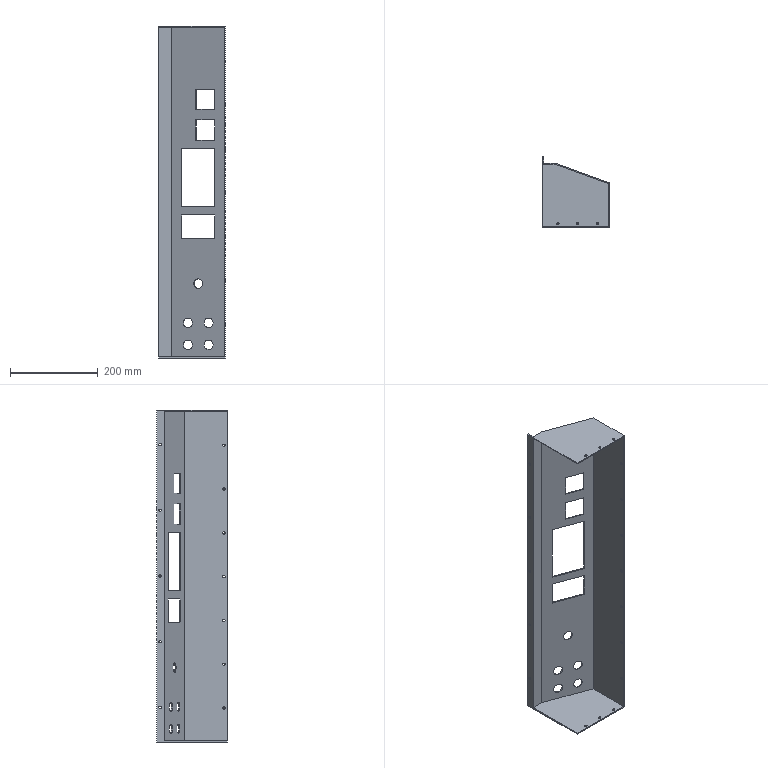Part | STEP file | MT-COMBO-119-S026 | 1 solid | 76 faces | box 152.5 x 160 x 758 mm | volume 557156 mm3 | cylinder 46 | plane 30 | commonest cylinder face diameters 5.5 x36 22 x10